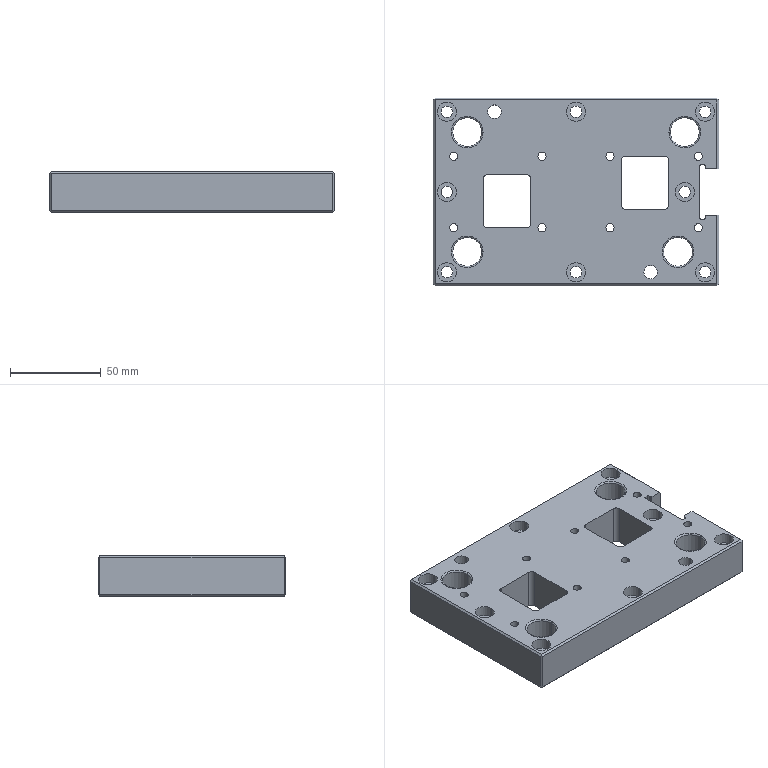Part | Creo | features DATUM PLANE 3, CURVE 2, CHAMFER 1, COORDINATE SYSTEM 1, CUT 1, PROTRUSION 1, ROUND 1 | 1 solid | 126 faces | box 157.5 x 103.5 x 22.5 mm | volume 294223 mm3 | cylinder 74 | plane 44 | torus 8 | commonest cylinder face diameters 4.5 x24 6.375 x16 10.5 x16 16 x8 1.5 x6 7.5 x4